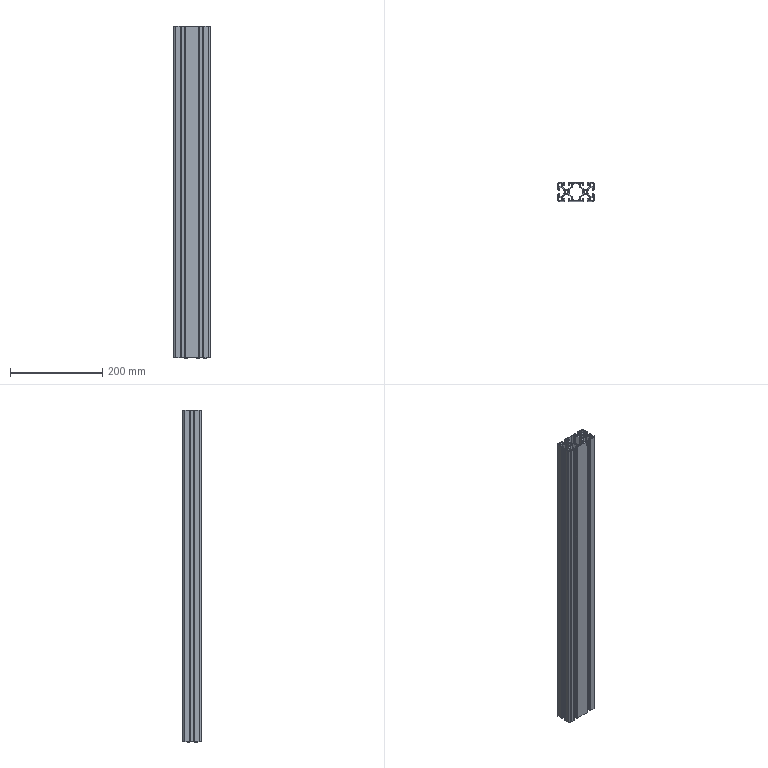Part | STEP file | LE-8-4080-S-OO_LE0307101856 | 1 solid | 286 faces | box 80 x 40 x 720 mm | volume 579034 mm3 | cylinder 144 | plane 142 | commonest cylinder face diameters 0.6 x48 2 x36 4 x28 0.4 x12 5 x4 6 x4